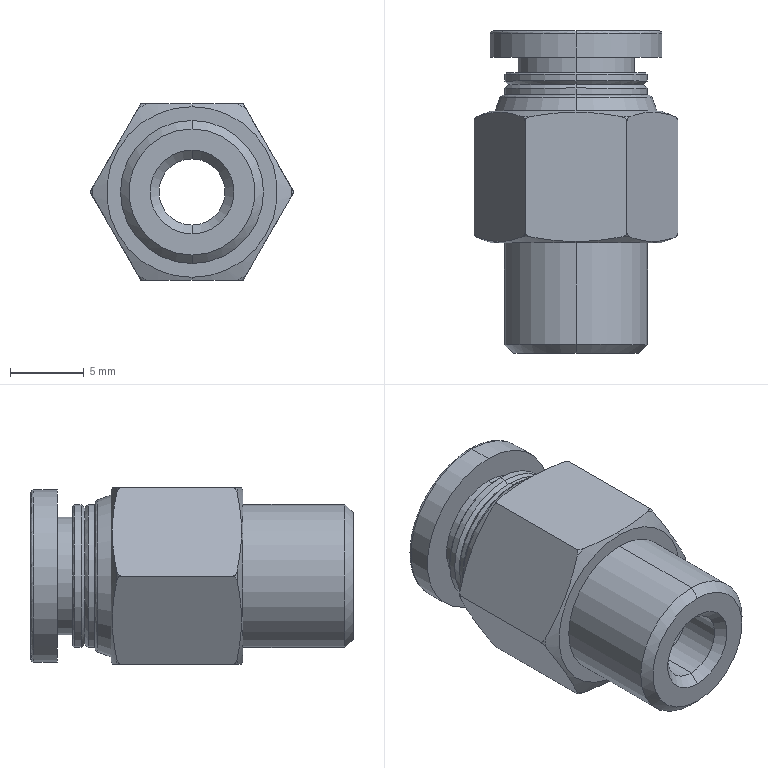Part | STEP file | 11-PC60111 | 1 solid | 62 faces | box 13.856 x 21.9 x 12 mm | volume 1535 mm3 | spline 18 | cone 16 | cylinder 14 | plane 14 | commonest cylinder face diameters 9.7 x4 4.5 x2 6 x2 8 x2 9.728 x2 11.7 x2